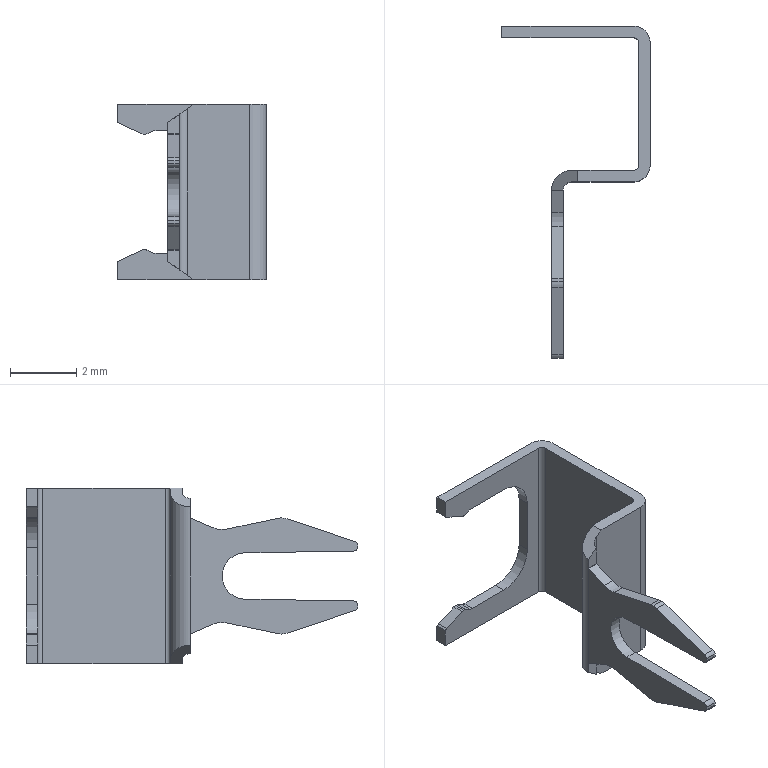Part | STEP file | Harpoon_Default | 1 solid | 63 faces | box 4.47 x 10 x 5.3 mm | volume 19.521 mm3 | plane 35 | cylinder 26 | spline 2 | commonest cylinder face diameters 0.3 x6 1 x5 1.4 x4 0.4 x3 0.494 x2 0.6 x2